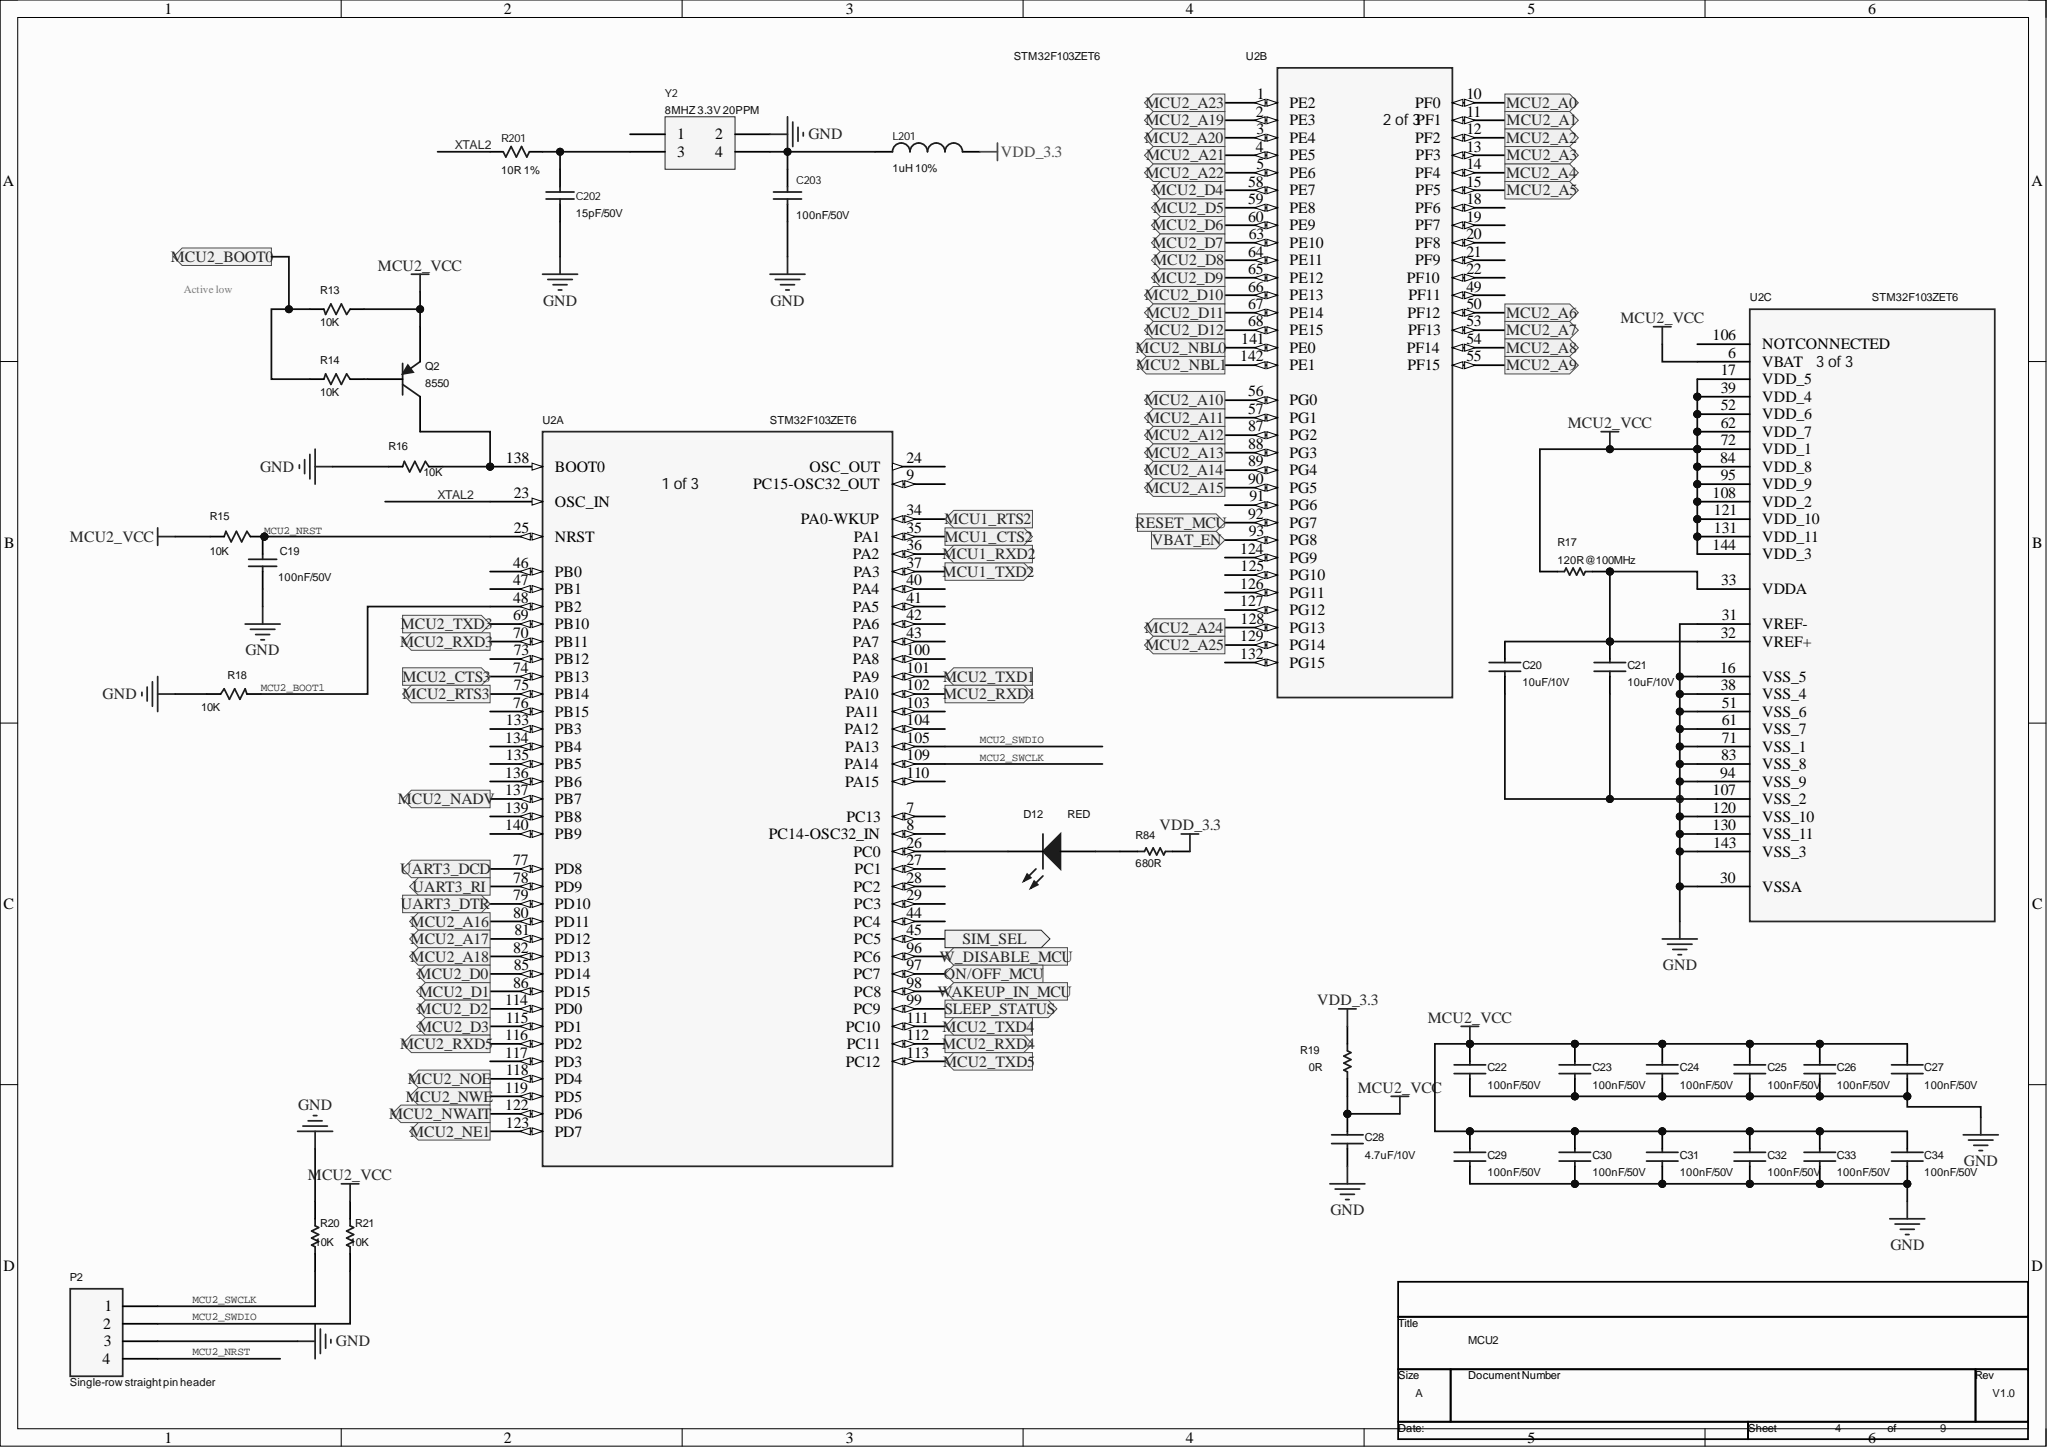Circuit board | Altium Designer | 313 parts | 216 nets | one sheet of the schematic
Parts on this sheet (reference | value | footprint):
C19 | 100nF/50V | 0603
C20 | 10uF/10V | C0603
C21 | 10uF/10V | C0603
C22 | 100nF/50V | C0603
C23 | 100nF/50V | C0603
C24 | 100nF/50V | C0603
C25 | 100nF/50V | C0603
C26 | 100nF/50V | C0603
C27 | 100nF/50V | C0603
C28 | 4.7uF/10V | C0805
C29 | 100nF/50V | C0603
C30 | 100nF/50V | C0603
C31 | 100nF/50V | C0603
C32 | 100nF/50V | C0603
C33 | 100nF/50V | C0603
C34 | 100nF/50V | C0603
C202 | 15pF/50V | C0603
C203 | 100nF/50V | C0603
D12 | RED | LED_0805
L201 | 1uH 10% | SMD_L6.0-W6.0
P2 | Single-row straight pin header | HDR1X4
Q2 | 8550 | SOT-23-SS8550
R13 | 10K | 0603
R14 | 10K | 0603
R15 | 10K | 0603
R16 | 10K | 0603
R17 | 120R@100MHz | 0603
R18 | 10K | 0603
R19 | 0R | 0603
R20 | 10K | 0603
R21 | 10K | 0603
R84 | NA | 0603
R201 | 10R 1% | R0805
U2 | STM32F103ZET6 | LQFP144-20x20mm
Y2 | 8MHZ 3.3V 20PPM | XTAL 5.7X7.0-SM - duplicate
Nets of these parts (net: part-pin ...):
XTAL2: R201-1 U2-23
VDD_3.3: L201-2 R19-1 R84-1
NetQ2_3: Q2-3 R16-2 U2-138
NetQ2_1: Q2-1 R14-1
NetP3_12: R13-1 R14-2
NetD12_2: D12-2 U2-26
NetD12_1: D12-1 R84-2
NetC203_1: C203-1 L201-1 Y2-4
NetC202_2: C202-2 R201-2 Y2-3
NetC20_1: C20-1 C21-1 R17-2 U2-32 U2-33
MCU2_VCC: C22-1 C23-1 C24-1 C25-1 C26-1 C27-1 C28-1 C29-1 C30-1 C31-1 C32-1 C33-1 C34-1 Q2-2 R13-2 R15-2 R17-1 R19-2 R21-2 U2-6 U2-17 U2-39 U2-52 U2-62 U2-72 U2-84 U2-95 U2-108 U2-121 U2-131 U2-144
MCU2_SWDIO: P2-2 R21-1 U2-105
MCU2_SWCLK: P2-1 R20-1 U2-109
MCU2_NRST: C19-2 P2-4 R15-1 U2-25
MCU2_BOOT1: R18-2 U2-48
GND: C19-1 C20-2 C21-2 C22-2 C23-2 C24-2 C25-2 C26-2 C27-2 C28-2 C29-2 C30-2 C31-2 C32-2 C33-2 C34-2 C202-1 C203-2 P2-3 R16-1 R18-1 R20-2 Y2-2 U2-16 U2-30 U2-31 U2-38 U2-51 U2-61 U2-71 U2-83 U2-94 U2-107 U2-120 U2-130 U2-143